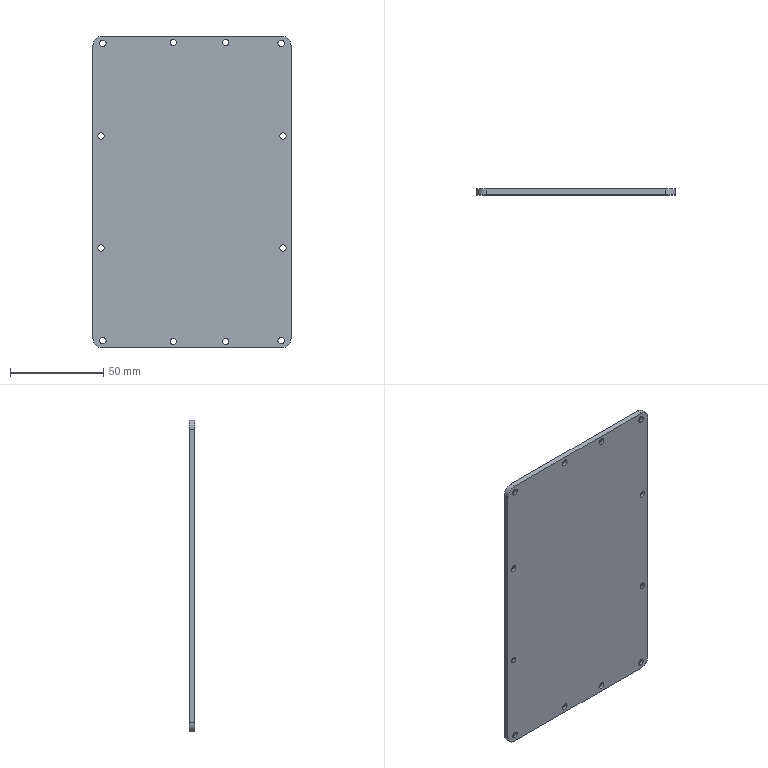Part | SolidWorks | features Extrusion 1, HoleWzd 1 | 1 solid | 58 faces | box 106 x 3 x 167 mm | volume 52528 mm3 | cylinder 28 | cone 24 | plane 6 | commonest cylinder face diameters 3.4 x24 10 x4